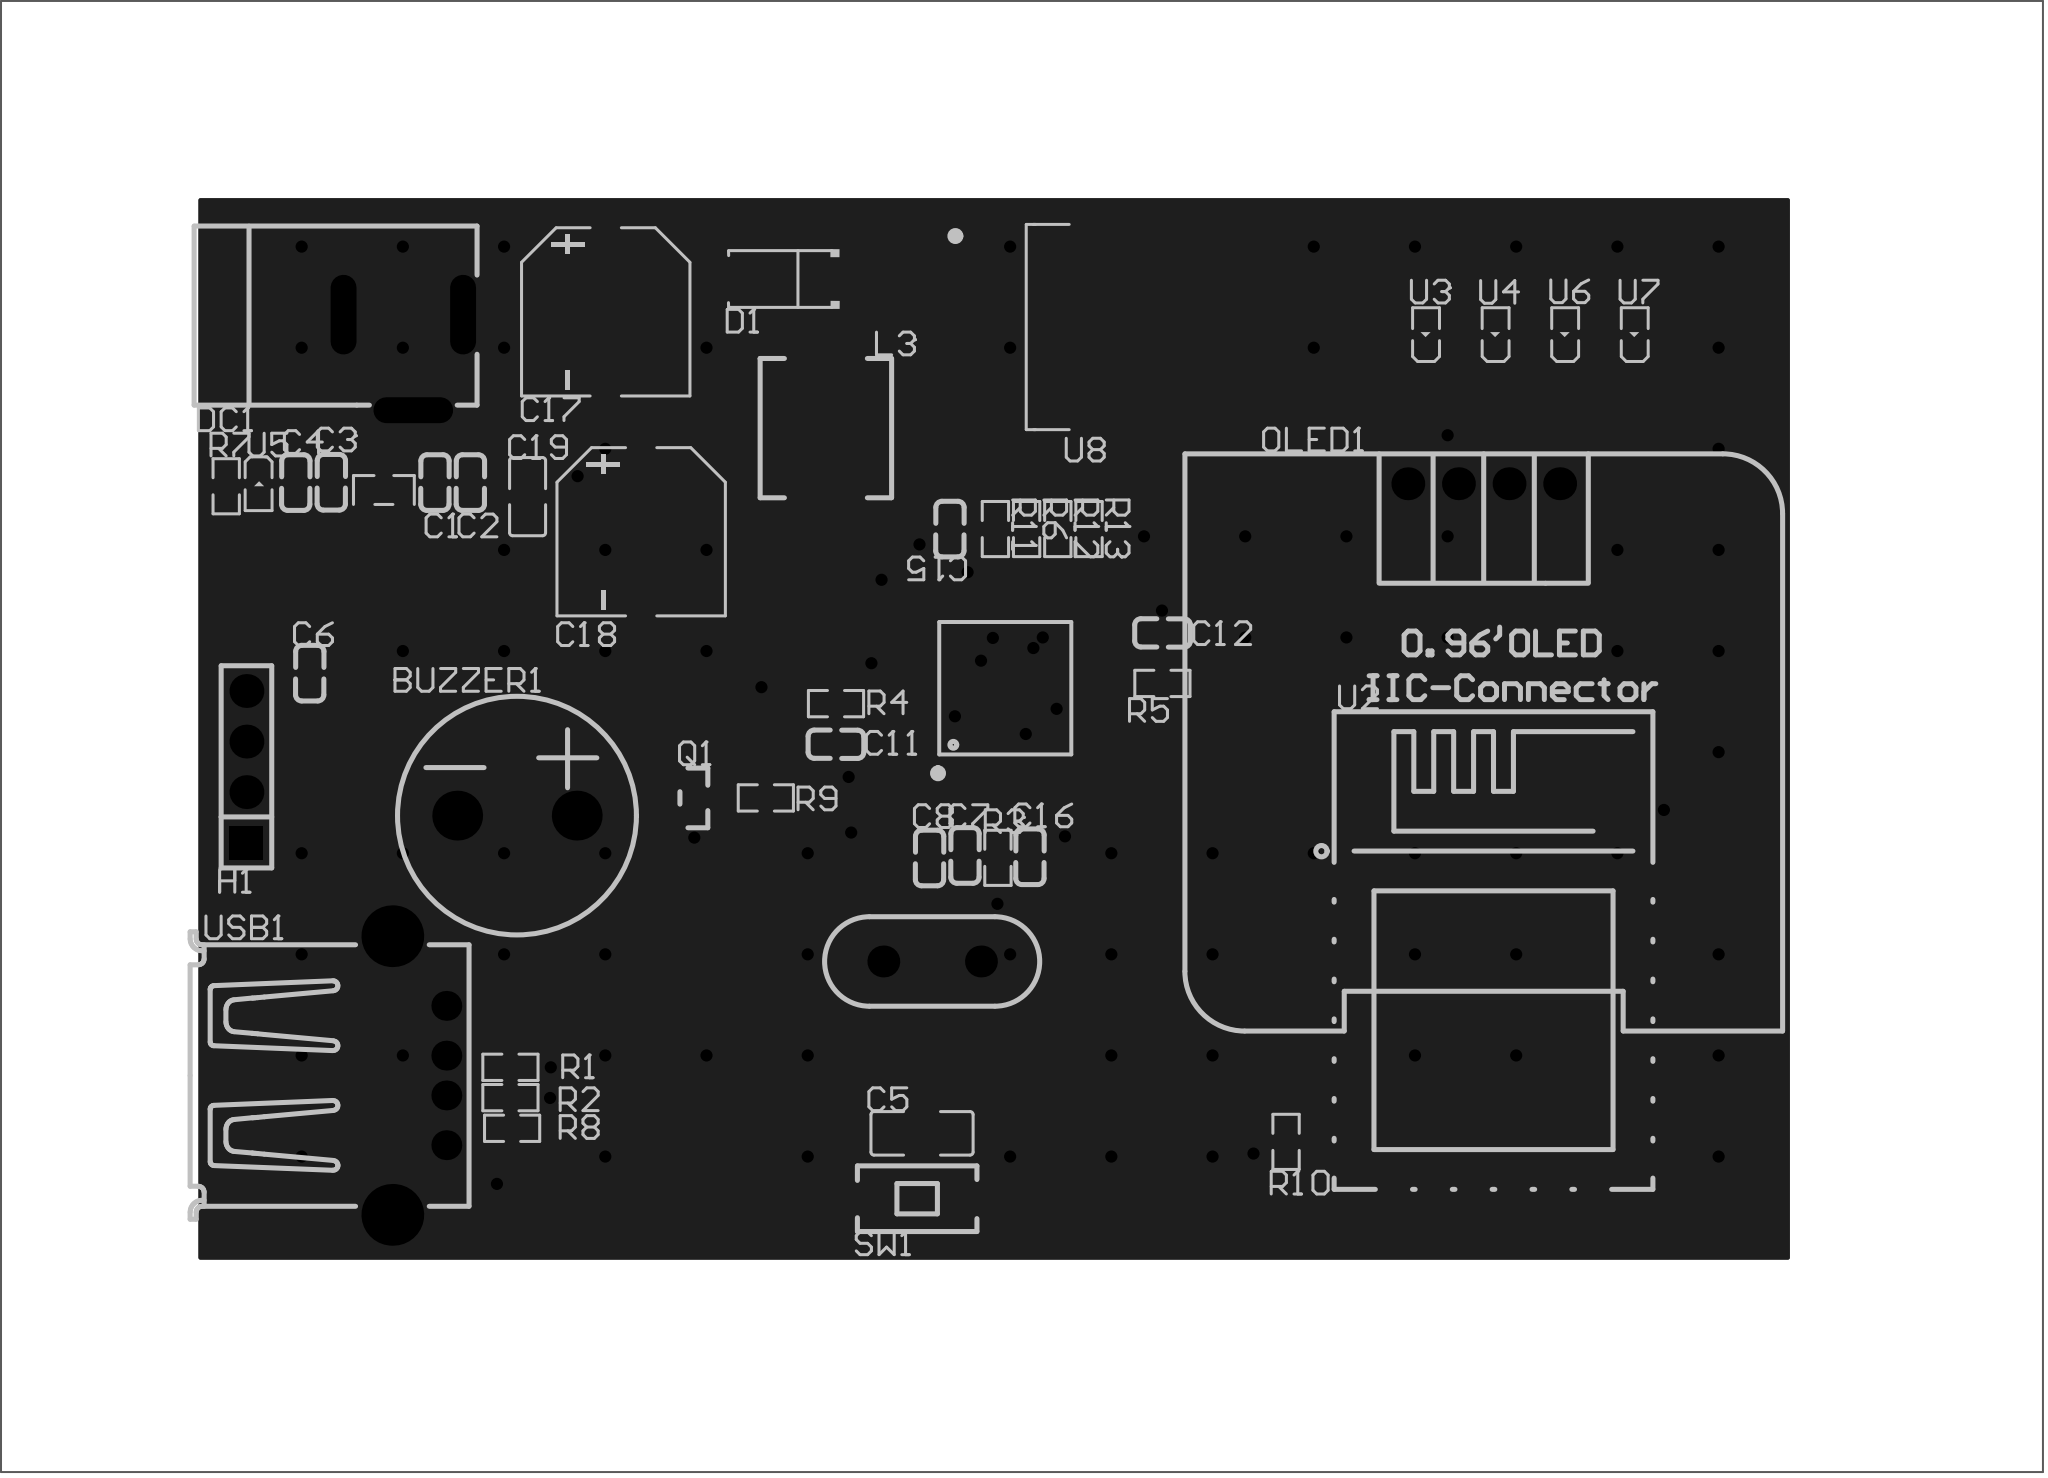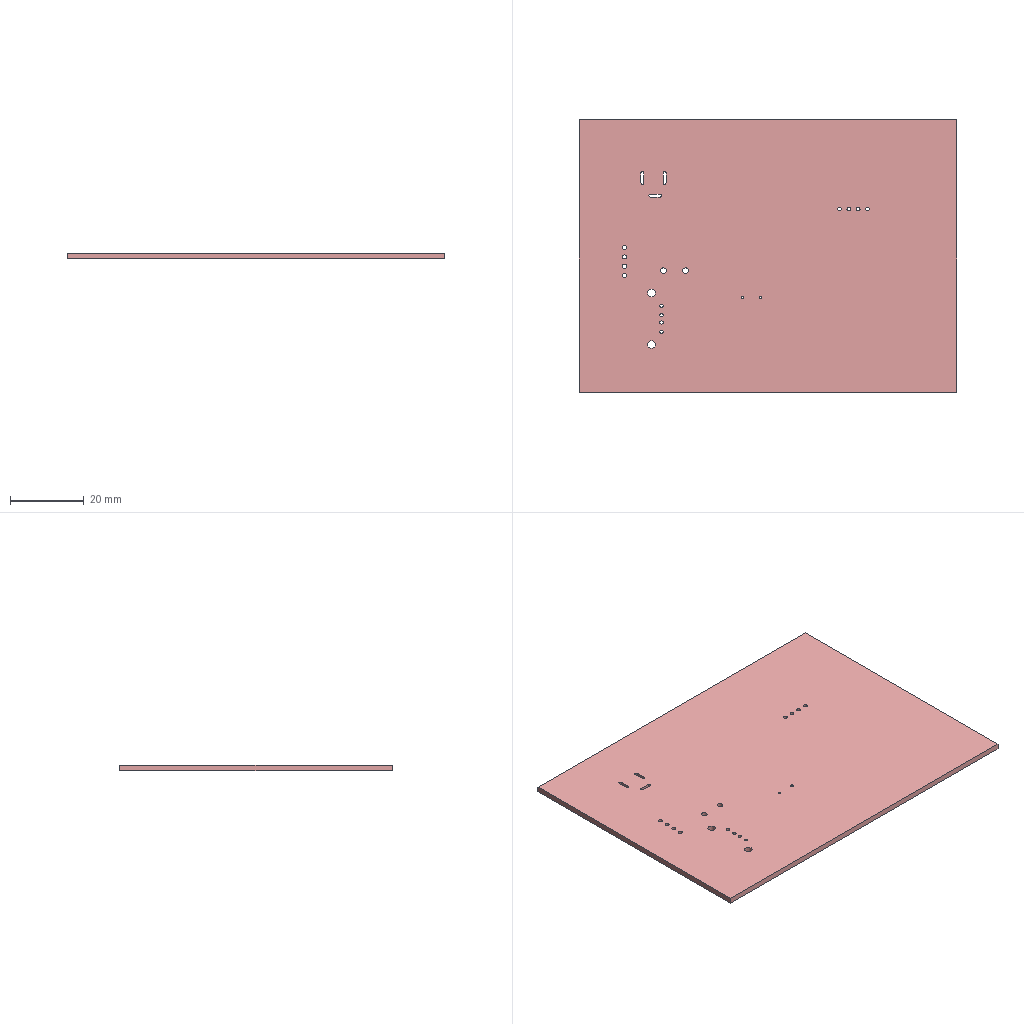Circuit board layout | Altium Designer | box 102.5 x 73.9 x 1.6 mm
Layer stack:
# Altium Designer layer stack of  (unit mm; dielectric type: 0 none, 1 core, 2 prepreg, 3 surface material)
index,name,kind,layer,copper_thickness_mm,dielectric_type,dielectric_thickness_mm,dielectric_material,dielectric_constant
0,Top Paste Mask Layer,other,,,,,,
1,Top Silkscreen Layer,other,,,,,,
2,Top Solder Mask Layer,dielectric,,,3,0.01,,3.3
3,Top Layer,copper,Top Layer,0.035,,,,
4,Dielectric1,dielectric,,,3,1.51,FR4,4.5
5,Bottom Layer,copper,Bottom Layer,0.035,,,,
6,Bottom Solder Mask Layer,dielectric,,,3,0.01,,3.3
7,Bottom Silkscreen Layer,other,,,,,,
8,Bottom Paste Mask Layer,other,,,,,,
# drill layer pairs: low layer,high layer
drill_pair,Top Layer,Bottom Layer
Part placement:
Designator,Comment,Layer,Footprint,Center-X(mm),Center-Y(mm),Rotation
U1,STM32F103C8T6,TopLayer,LQFP-48_L7.0-W7.0-P0.50-LS9.0-BL,120.269,109.22,0
LDO1,SC662K-3.3V,TopLayer,SOT-23-3_L2.9-W1.3-P1.90-LS2.4-BR,89.068,119.192,270
C1,10uF,TopLayer,C0603,91.633,119.573,90
C4,10uF,TopLayer,C0603,84.642,119.558,270
C2,100nF,TopLayer,C0603,93.411,119.573,90
C3,100nF,TopLayer,C0603,86.426,119.573,270
R1,20Ω,TopLayer,R0603,95.419,90.186,0
R2,20Ω,TopLayer,R0603,95.419,88.662,0
R3,1kΩ,TopLayer,R0603,119.888,100.711,270
SW1,TS-1101-C-W,TopLayer,SW-SMD_L6.0-W3.3-LS8.0,115.697,83.566,180
C5,100uF,TopLayer,C1206,116.078,86.868,180
C6,100nF,TopLayer,C0603,85.344,109.982,270
R5,10kΩ,TopLayer,R0603,128.143,109.474,180
R4,10kΩ,TopLayer,R0603,111.76,108.458,0
X1,8MHz,TopLayer,OSC-TH_L10.0-W4.5-P5.00,116.586,95.504,90
C7,20pF,TopLayer,C0603,118.237,100.838,90
C8,20pF,TopLayer,C0603,116.459,100.711,90
U5,42-51/GHC-YW2X2K/3T,TopLayer,LED-SMD_L1.6-W0.8-FD_GREEN-1,82.804,119.507,90
R7,510Ω,TopLayer,R0603,81.153,119.38,270
C11,100nF,TopLayer,C0603,111.765,106.416,0
C12,100nF,TopLayer,C0603,128.143,112.014,180
C15,100nF,TopLayer,C0603,117.475,117.221,270
C16,4.7nF,TopLayer,C0603,121.498,100.773,90
R8,1.5kΩ,TopLayer,R0603,95.504,87.122,0
BUZZER1,buzzer,TopLayer,BUZ-TH_BD12.0-P6.00-D0.9-RD,95.747,102.832,0
C17,,TopLayer,CAP-SMD_BD8.0-L8.3-W8.3-RD,100.203,128.143,90
C18,,TopLayer,CAP-SMD_BD8.0-L8.3-W8.3-RD,101.981,117.094,90
C19,,TopLayer,C0805,96.28,118.858,270
D1,,TopLayer,SMA_L4.3-W2.6-LS5.2-RD,108.966,129.794,180
DC1,,TopLayer,DC-2.0,90.043,125.603,180
L3,,TopLayer,IND-SMD_L7.0-W6.6,111.252,122.301,270
OLED1,,TopLayer,0.96OLED_4P,144.272,119.507,0
Q1,,TopLayer,S8050_SOT-23,104.627,103.721,180
R6,510Ω,TopLayer,R0603,121.327,117.23,270
R9,10K,TopLayer,R0603,108.238,103.721,180
R10,10K,TopLayer,R0603,134.349,86.44,90
R11,510Ω,TopLayer,R0603,119.761,117.23,270
R12,510Ω,TopLayer,R0603,122.894,117.23,270
R13,510Ω,TopLayer,R0603,124.46,117.23,270
U2,ESP8266,TopLayer,WIFIM-SMD_ESP-12F-ESP8266MOD,144.763,91.901,270
U3,42-51/GHC-YW2X2K/3T,TopLayer,LED-SMD_L1.6-W0.8-FD_GREEN-1,141.351,127,270
U4,42-51/GHC-YW2X2K/3T,TopLayer,LED-SMD_L1.6-W0.8-FD_GREEN-1,144.842,127,270
U6,42-51/GHC-YW2X2K/3T,TopLayer,LED-SMD_L1.6-W0.8-FD_GREEN-1,148.333,127,270
U7,42-51/GHC-YW2X2K/3T,TopLayer,LED-SMD_L1.6-W0.8-FD_GREEN-1,151.825,127,270
U8,LM2596S-5.0,TopLayer,TO-263-5_L10.2-W8.9-P1.70-BR,122.809,127.381,180
USB1,,TopLayer,USB__Type-A,90.847,89.773,270
H1,,TopLayer,HDR-TH_4P-P2.54-V-M,82.169,105.283,90
Pad and via stacks:
# Altium Designer via and pad stacks of  (unit mm). Each distinct definition once, with the count of objects using it.
# via: kind,start_layer,end_layer,hole_mm,diameter_mm,mode(0 simple;1 top-mid-bottom;2 full stack),diameter_per_layer,count,example_net
# pad: kind,layer,hole_mm,hole_type(0 round;1 square;2 slot),plating,top_size,top_shape(1 round;2 rect;3 octagon;9 rounded rect),mid_size,bottom_size,mode,footprint,size_per_layer,count,example
pad,Top Layer,0,0,plated,0.27x1.5,1,0.27x1.5,0.27x1.5,0,LQFP-48_L7.0-W7.0-P0.50-LS9.0-BL,,24,U1.1
pad,Top Layer,0,0,plated,1.5x0.27,1,1.5x0.27,1.5x0.27,0,LQFP-48_L7.0-W7.0-P0.50-LS9.0-BL,,24,U1.13
pad,Top Layer,0,0,plated,1.25x0.7,2,1.25x0.7,1.25x0.7,0,SOT-23-3_L2.9-W1.3-P1.90-LS2.4-BR,,3,LDO1.1
pad,Top Layer,0,0,plated,0.8x0.9,2,0.8x0.9,0.8x0.9,0,C0603,,22,C1.2
pad,Top Layer,0,0,plated,0.8065x0.864,2,0.8065x0.864,0.8065x0.864,0,R0603,,26,R1.2
pad,Top Layer,0,0,plated,1.9x1.5,2,1.9x1.5,1.9x1.5,0,SW-SMD_L6.0-W3.3-LS8.0,,2,SW1.1
pad,Top Layer,0,0,plated,1.485x1.728,2,1.485x1.728,1.485x1.728,0,C1206,,2,C5.2
pad,Top Layer,0,0,plated,0.8x0.7,2,0.8x0.7,0.8x0.7,0,LED-SMD_L1.6-W0.8-FD_GREEN-1,,10,U5.1
pad,Top Layer,0,0,plated,3.61x1.26,2,3.61x1.26,3.61x1.26,0,CAP-SMD_BD8.0-L8.3-W8.3-RD,,4,C17.1
pad,Top Layer,0,0,plated,1.41x1.35,2,1.41x1.35,1.41x1.35,0,C0805,,2,C19.2
pad,Top Layer,0,0,plated,2x2,2,2x2,2x2,0,SMA_L4.3-W2.6-LS5.2-RD,,2,D1.2
pad,Top Layer,0,0,plated,2.799x3.701,2,2.799x3.701,2.799x3.701,0,IND-SMD_L7.0-W6.6,,2,L3.1
pad,Top Layer,0,0,plated,1x0.8,2,1x0.8,1x0.8,0,S8050_SOT-23,,3,Q1.2
pad,Top Layer,0,0,plated,2.5x1.4,2,2.5x1.4,2.5x1.4,0,WIFIM-SMD_ESP-12F-ESP8266MOD,,16,U2.16
pad,Top Layer,0,0,plated,1.7x1.4,2,1.7x1.4,1.7x1.4,0,WIFIM-SMD_ESP-12F-ESP8266MOD,,6,U2.22
pad,Top Layer,0,0,plated,3.083x1.02,2,3.083x1.02,3.083x1.02,0,TO-263-5_L10.2-W8.9-P1.70-BR,,5,U8.1
pad,Top Layer,0,0,plated,8.5x11,2,8.5x11,8.5x11,0,TO-263-5_L10.2-W8.9-P1.70-BR,,1,U8.6
pad,Multi-Layer,0.7,0,plated,1.6x1.6,1,1.6x1.6,1.6x1.6,0,OSC-TH_L10.0-W4.5-P5.00,,2,X1.2
pad,Multi-Layer,1.5,0,plated,2.5x2.5,1,2.5x2.5,2.5x2.5,0,BUZ-TH_BD12.0-P6.00-D0.9-RD,,2,BUZZER1.1
pad,Multi-Layer,0.8001,2,plated,4x1.3,1,4x1.3,4x1.3,0,DC-2.0,,3,DC1.2
pad,Multi-Layer,1,0,plated,1.65x1.65,1,1.65x1.65,1.65x1.65,0,0.96OLED_4P,,4,OLED1.4
pad,Multi-Layer,2.1,0,plated,3.1x3.1,1,3.1x3.1,3.1x3.1,0,USB_ Type-A,,2,USB1.SH2
pad,Multi-Layer,0.9,0,plated,1.5x1.5,1,1.5x1.5,1.5x1.5,0,USB_ Type-A,,4,USB1.1
pad,Multi-Layer,1.1,0,plated,1.7x1.7,2,1.7x1.7,1.7x1.7,0,HDR-TH_4P-P2.54-V-M,,1,H1.1
pad,Multi-Layer,1.1,0,plated,1.7x1.7,1,1.7x1.7,1.7x1.7,0,HDR-TH_4P-P2.54-V-M,,3,H1.2
via,Top Layer,Bottom Layer,0.3048,0.61,0,,100,PA12
Copper pours:
name,layer,net,type(0 solid;1 hatched;2 none)
Top Layer-GND,Top Layer,GND,0
Bottom Layer-GND,Bottom Layer,GND,0
Design rules, without the lines most boards share:
# Altium Designer design rules of  (exported by Altium Designer, unit mm)
# columns: name | kind | enabled | priority | scope1 | scope2 | descriptor | typed fields (field=value)
otherClearance | 52 | enabled | 1 | All | All | Hole To Hole Clearance (Gap=11.8mil) (All),(All) | gap=0.2997